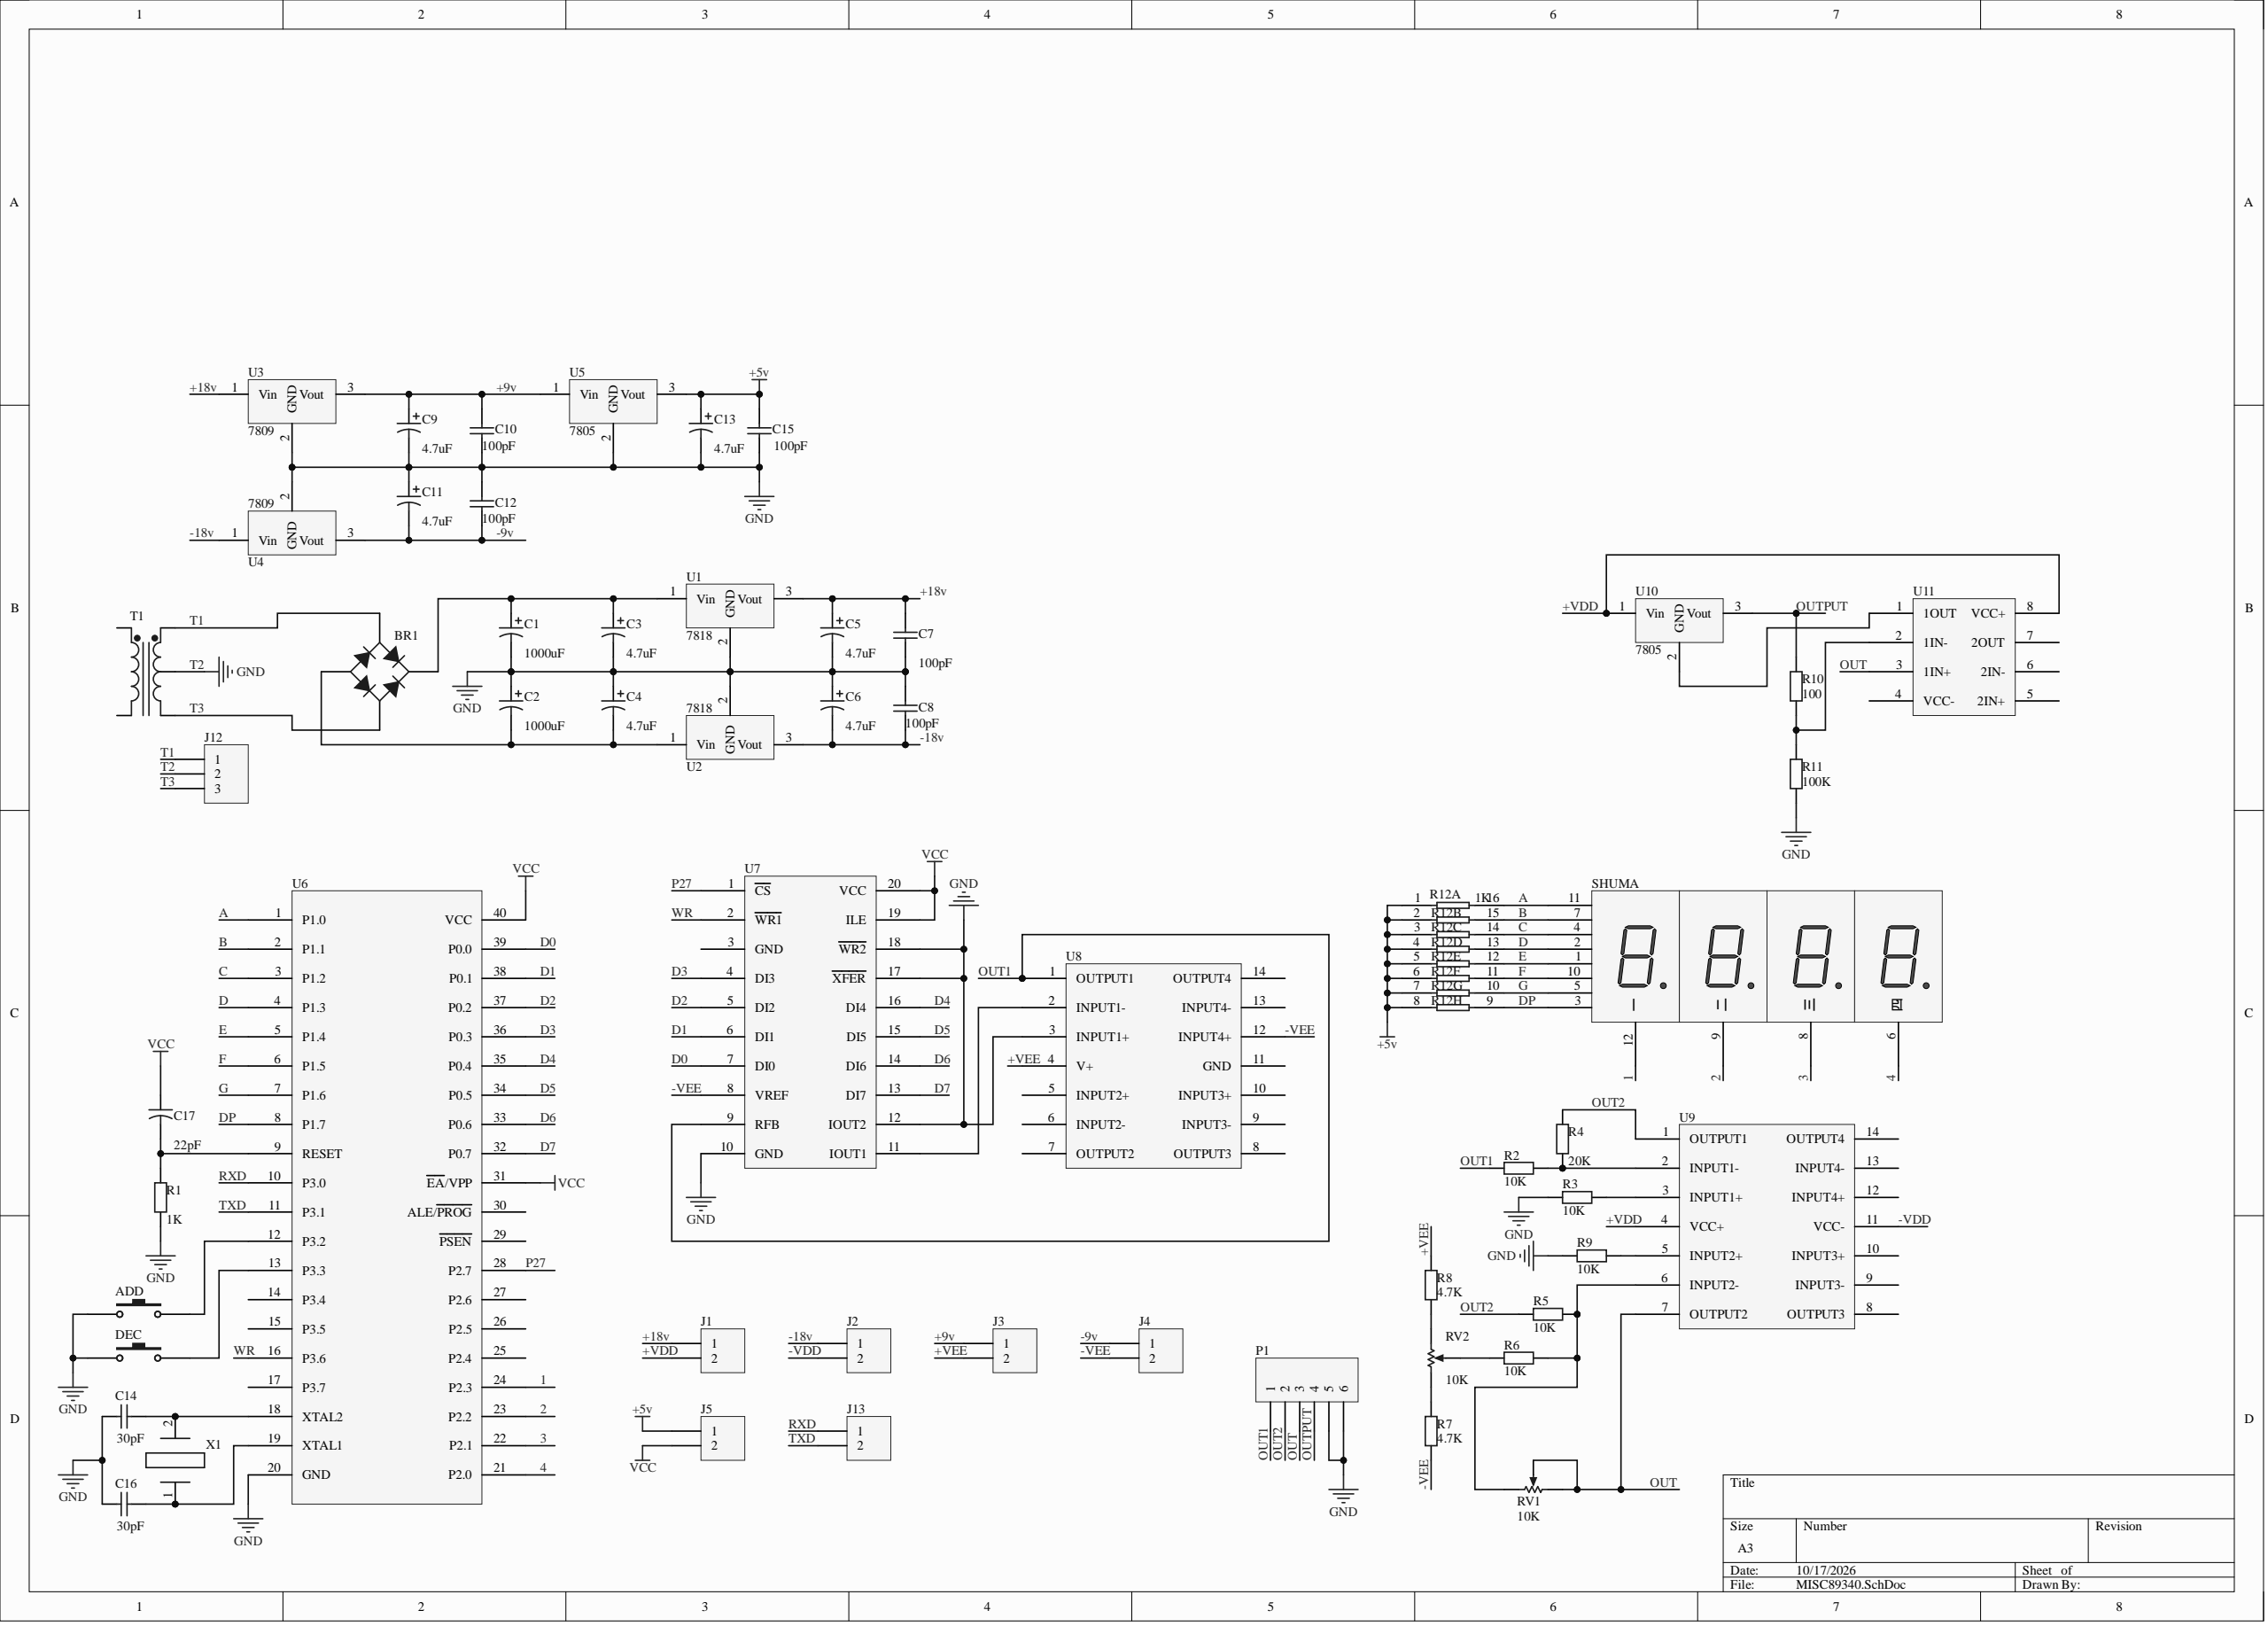Circuit board | Altium Designer | 56 parts | 58 nets
Bill of materials:
Comment,Description,Designator,Footprint,LibRef,Quantity
"SW-PB","Switch","ADD, DEC","SPST-2","SW-PB","2"
"Bridge1","Full Wave Diode Bridge","BR1","LC-KBP","Bridge1","1"
"Cap Pol1","Polarized Capacitor (Radial)","C1, C2, C3, C4, C5, C6, C9, C11, C13","RB7.6-15","Cap Pol1","9"
"Cap","Capacitor","C7, C8, C10, C12, C14, C15, C16","RAD-0.3","Cap","7"
"Cap2","Capacitor","C17","CAPR5-4X5","Cap2","1"
"Header 2","Header, 2-Pin","J1, J2, J3, J4, J5, J13","HDR1X2","Header 2","6"
"Header 3","Header, 3-Pin","J12","HDR1X3","Header 3","1"
"Header 6","Header, 6-Pin","P1","HDR1X6","Header 6","1"
"Res2","Resistor","R1, R2, R3, R4, R5, R6, R7, R8, R9, R10, R11","AXIAL-0.4","Res2","11"
"Res Pack2","Isolated Resistor Network - Parts","R12","DIP-16","Res Pack2","1"
"RPot","Potentiometer","RV1, RV2","VR5","RPot","2"
"Dpy Red-CA","7.62 mm Black Surface HER 7-Segment Display: CA, RH DP","SHUMA","四位数码管","Dpy Red-CA","1"
"Trans CT","Center-Tapped Transformer (Coupled Inductor Model)","T1","TRF_5","Trans CT","1"
"7818","Voltage Regulator","U1, U2","7805","Volt Reg","2"
"7809","Voltage Regulator","U3, U4","7805","Volt Reg","2"
"7805","Voltage Regulator","U5, U10","7805","Volt Reg","2"
"89c51","","U6","89c51","Component_1","1"
"Component_1","","U7","DAC0832","Component_1","1"
"Component_1","","U8","LM324","Component_1","1"
"Component_1","","U9","TL084","Component_1","1"
"","","U11","NE5532","Component_1","1"
"Component_1","","X1","LC-HC-49S","Component_1","1"
Netlist (Protel format):
[
ADD
SPST-2
SW-PB



]
[
BR1
LC-KBP
Bridge1



]
[
C1
RB7.6-15
Cap Pol1



]
[
C2
RB7.6-15
Cap Pol1



]
[
C3
RB7.6-15
Cap Pol1



]
[
C4
RB7.6-15
Cap Pol1



]
[
C5
RB7.6-15
Cap Pol1



]
[
C6
RB7.6-15
Cap Pol1



]
[
C7
RAD-0.3
Cap



]
[
C8
RAD-0.3
Cap



]
[
C9
RB7.6-15
Cap Pol1



]
[
C10
RAD-0.3
Cap



]
[
C11
RB7.6-15
Cap Pol1



]
[
C12
RAD-0.3
Cap



]
[
C13
RB7.6-15
Cap Pol1



]
[
C14
RAD-0.3
Cap



]
[
C15
RAD-0.3
Cap



]
[
C16
RAD-0.3
Cap



]
[
C17
CAPR5-4X5
Cap2



]
[
DEC
SPST-2
SW-PB



]
[
J1
HDR1X2
Header 2



]
[
J2
HDR1X2
Header 2



]
[
J3
HDR1X2
Header 2



]
[
J4
HDR1X2
Header 2



]
[
J5
HDR1X2
Header 2



]
[
J12
HDR1X3
Header 3



]
[
J13
HDR1X2
Header 2



]
[
P1
HDR1X6
Header 6



]
[
R1
AXIAL-0.4
Res2



]
[
R2
AXIAL-0.4
Res2



]
[
R3
AXIAL-0.4
Res2



]
[
R4
AXIAL-0.4
Res2



]
[
R5
AXIAL-0.4
Res2



]
[
R6
AXIAL-0.4
Res2



]
[
R7
AXIAL-0.4
Res2



]
[
R8
AXIAL-0.4
Res2



]
[
R9
AXIAL-0.4
Res2



]
[
R10
AXIAL-0.4
Res2



]
[
R11
AXIAL-0.4
Res2



]
[
R12
DIP-16
Res Pack2



]
[
RV1
VR5
RPot



]
[
RV2
VR5
RPot



]
[
SHUMA
四位数码管
Dpy Red-CA



]
[
T1
TRF_5
Trans CT



]
[
U1
7805
7818



]
[
U2
7805
7818



]
[
U3
7805
7809



]
[
U4
7805
7809



]
[
U5
7805
7805



]
[
U6
89c51
89c51



]
[
U7
DAC0832
Component_1



]
[
U8
LM324
Component_1



]
[
U9
TL084
Component_1



]
[
U10
7805
7805



]
[
U11
NE5532




]
[
X1
LC-HC-49S
Component_1



]
(
WR
U6-16
U7-2
)
(
VCC
C17-1
J5-2
U6-31
U6-40
U7-19
U7-20
)
(
TXD
J13-2
U6-11
)
(
T3
BR1-2
J12-3
T1-5
)
(
T2
ADD-1
C1-2
C2-1
C3-2
C4-1
C5-2
C6-1
C7-1
C8-2
C9-2
C10-1
C11-1
C12-2
C13-2
C14-1
C15-1
C16-1
DEC-1
J12-2
P1-5
P1-6
R1-1
R3-2
R9-2
R11-2
T1-4
U1-2
U2-2
U3-2
U4-2
U5-2
U6-20
U7-10
U7-12
U7-17
U7-18
U8-3
)
(
T1
BR1-4
J12-1
T1-3
)
(
RXD
J13-1
U6-10
)
(
P27
U6-28
U7-1
)
(
OUTPUT
P1-4
R10-1
U10-3
)
(
OUT2
P1-2
R4-2
R5-2
U9-1
)
(
OUT1
P1-1
R2-2
U7-9
U8-1
)
(
OUT
P1-3
RV1-1
RV1-3
U9-7
U11-3
)
(
NetU10_2
U10-2
U11-1
)
(
NetU7_11
U7-11
U8-2
)
(
NetR10_2
R10-2
R11-1
U11-2
)
(
NetR9_1
R9-1
U9-5
)
(
NetR8_2
R8-2
RV2-2
)
(
NetR7_1
R7-1
RV2-1
)
(
NetR6_2
R6-2
RV2-3
)
(
NetR5_1
R5-1
R6-1
RV1-2
U9-6
)
(
NetR3_1
R3-1
U9-3
)
(
NetR2_1
R2-1
R4-1
U9-2
)
(
NetDEC_2
DEC-2
U6-13
)
(
NetC17_2
C17-2
R1-2
U6-9
)
(
NetC16_2
C16-2
U6-19
X1-1
)
(
NetC14_2
C14-2
U6-18
X1-2
)
(
NetBR1_3
BR1-3
C2-2
C4-2
U2-1
)
(
NetBR1_1
BR1-1
C1-1
C3-1
U1-1
)
(
NetADD_2
ADD-2
U6-12
)
(
G
R12-10
SHUMA-5
U6-7
)
(
F
R12-11
SHUMA-10
U6-6
)
(
E
R12-12
SHUMA-1
U6-5
)
(
DP
R12-9
SHUMA-3
U6-8
)
(
D7
U6-32
U7-13
)
(
D6
U6-33
U7-14
)
(
D5
U6-34
U7-15
)
(
D4
U6-35
U7-16
)
(
D3
U6-36
U7-4
)
(
D2
U6-37
U7-5
)
(
D1
U6-38
U7-6
)
(
D0
U6-39
U7-7
)
(
D
R12-13
SHUMA-2
U6-4
)
(
C
R12-14
SHUMA-4
U6-3
)
(
B
R12-15
SHUMA-7
U6-2
)
(
A
R12-16
SHUMA-11
U6-1
)
(
-VEE
J4-2
R7-2
U7-8
U8-12
)
(
-VDD
J2-2
U9-11
)
(
-18v
C6-2
C8-1
J2-1
U2-3
U4-1
)
(
-9v
C11-2
C12-1
J4-1
U4-3
)
(
+VEE
J3-2
R8-1
U8-4
)
(
+VDD
J1-2
U9-4
U10-1
U11-8
)
(
+18v
C5-1
C7-2
J1-1
U1-3
U3-1
)
(
+9v
C9-1
C10-2
J3-1
U3-3
U5-1
)
(
+5v
C13-1
C15-2
J5-1
R12-1
R12-2
R12-3
R12-4
R12-5
R12-6
R12-7
R12-8
U5-3
)
(
4
SHUMA-6
U6-21
)
(
3
SHUMA-8
U6-22
)
(
2
SHUMA-9
U6-23
)
(
1
SHUMA-12
U6-24
)